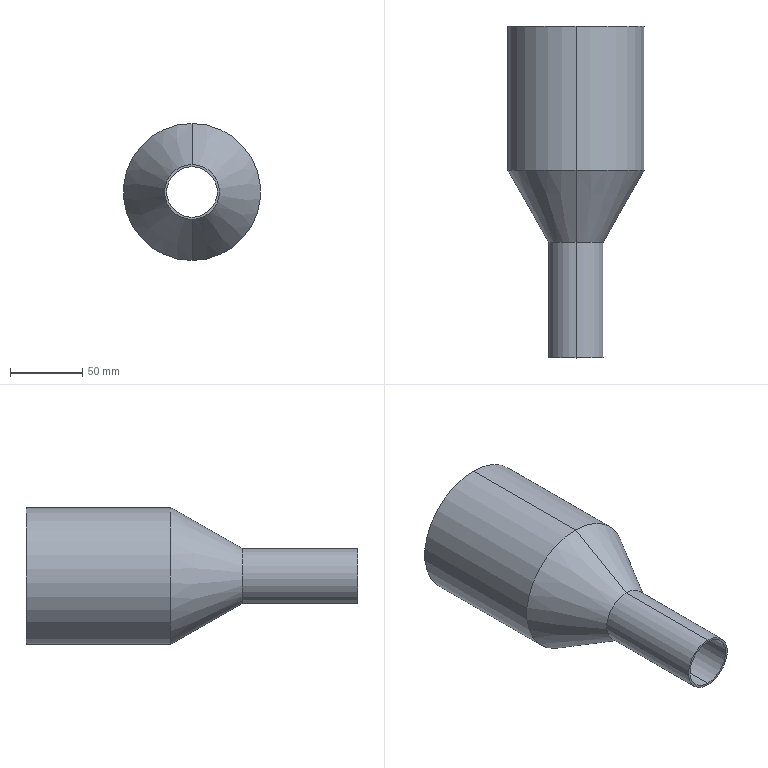Part | SolidWorks | features BaseBody 1 | 1 solid | 14 faces | box 95 x 230 x 95 mm | volume 75396 mm3 | cylinder 8 | cone 4 | plane 2 | commonest cylinder face diameters 35 x2 38 x2 92 x2 95 x2
STEP:
#1=CARTESIAN_POINT('',(0.,130.,47.5));
#2=VERTEX_POINT('',#1);
#3=CARTESIAN_POINT('',(0.,130.,-47.5));
#4=VERTEX_POINT('',#3);
#5=CARTESIAN_POINT('',(0.,130.,0.));
#6=DIRECTION('',(0.,1.,0.));
#7=DIRECTION('',(0.,0.,1.));
#8=AXIS2_PLACEMENT_3D('',#5,#6,#7);
#9=CIRCLE('',#8,47.5);
#10=EDGE_CURVE('',#2,#4,#9,.T.);
#11=ORIENTED_EDGE('',*,*,#10,.T.);
#12=CARTESIAN_POINT('',(0.,230.,-47.5));
#13=VERTEX_POINT('',#12);
#14=CARTESIAN_POINT('',(0.,119.95,-47.5));
#15=DIRECTION('',(0.,1.,0.));
#16=VECTOR('',#15,1000.);
#17=LINE('',#14,#16);
#18=EDGE_CURVE('',#4,#13,#17,.T.);
#19=ORIENTED_EDGE('',*,*,#18,.T.);
#20=CARTESIAN_POINT('',(0.,230.,47.5));
#21=VERTEX_POINT('',#20);
#22=CARTESIAN_POINT('',(0.,230.,0.));
#23=DIRECTION('',(0.,1.,0.));
#24=DIRECTION('',(0.,0.,1.));
#25=AXIS2_PLACEMENT_3D('',#22,#23,#24);
#26=CIRCLE('',#25,47.5);
#27=EDGE_CURVE('',#21,#13,#26,.T.);
#28=ORIENTED_EDGE('',*,*,#27,.F.);
#29=CARTESIAN_POINT('',(0.,119.95,47.5));
#30=DIRECTION('',(0.,1.,0.));
#31=VECTOR('',#30,1000.);
#32=LINE('',#29,#31);
#33=EDGE_CURVE('',#2,#21,#32,.T.);
#34=ORIENTED_EDGE('',*,*,#33,.F.);
#35=EDGE_LOOP('',(#11,#19,#28,#34));
#36=FACE_OUTER_BOUND('',#35,.T.);
#37=CARTESIAN_POINT('',(0.,119.95,0.));
#38=DIRECTION('',(0.,1.,0.));
#39=DIRECTION('',(0.,0.,1.));
#40=AXIS2_PLACEMENT_3D('',#37,#38,#39);
#41=CYLINDRICAL_SURFACE('',#40,47.5);
#42=ADVANCED_FACE('',(#36),#41,.T.);
#43=CARTESIAN_POINT('',(0.,80.,19.));
#44=VERTEX_POINT('',#43);
#45=CARTESIAN_POINT('',(0.,80.,-19.));
#46=VERTEX_POINT('',#45);
#47=CARTESIAN_POINT('',(0.,80.,0.));
#48=DIRECTION('',(0.,1.,0.));
#49=DIRECTION('',(0.,0.,1.));
#50=AXIS2_PLACEMENT_3D('',#47,#48,#49);
#51=CIRCLE('',#50,19.);
#52=EDGE_CURVE('',#44,#46,#51,.T.);
#53=ORIENTED_EDGE('',*,*,#52,.T.);
#54=CARTESIAN_POINT('',(0.,80.,-19.));
#55=DIRECTION('',(0.,0.8688,-0.4952));
#56=VECTOR('',#55,1000.);
#57=LINE('',#54,#56);
#58=EDGE_CURVE('',#46,#4,#57,.T.);
#59=ORIENTED_EDGE('',*,*,#58,.T.);
#60=ORIENTED_EDGE('',*,*,#10,.F.);
#61=CARTESIAN_POINT('',(0.,80.,19.));
#62=DIRECTION('',(0.,0.8688,0.4952));
#63=VECTOR('',#62,1000.);
#64=LINE('',#61,#63);
#65=EDGE_CURVE('',#44,#2,#64,.T.);
#66=ORIENTED_EDGE('',*,*,#65,.F.);
#67=EDGE_LOOP('',(#53,#59,#60,#66));
#68=FACE_OUTER_BOUND('',#67,.T.);
#69=CARTESIAN_POINT('',(0.,80.,0.));
#70=DIRECTION('',(0.,1.,0.));
#71=DIRECTION('',(0.,0.,1.));
#72=AXIS2_PLACEMENT_3D('',#69,#70,#71);
#73=CONICAL_SURFACE('',#72,19.,0.5181);
#74=ADVANCED_FACE('',(#68),#73,.T.);
#75=CARTESIAN_POINT('',(0.,0.,19.));
#76=VERTEX_POINT('',#75);
#77=CARTESIAN_POINT('',(0.,0.,-19.));
#78=VERTEX_POINT('',#77);
#79=CARTESIAN_POINT('',(0.,0.,0.));
#80=DIRECTION('',(0.,1.,0.));
#81=DIRECTION('',(0.,0.,1.));
#82=AXIS2_PLACEMENT_3D('',#79,#80,#81);
#83=CIRCLE('',#82,19.);
#84=EDGE_CURVE('',#76,#78,#83,.T.);
#85=ORIENTED_EDGE('',*,*,#84,.T.);
#86=CARTESIAN_POINT('',(0.,119.95,-19.));
#87=DIRECTION('',(0.,1.,0.));
#88=VECTOR('',#87,1000.);
#89=LINE('',#86,#88);
#90=EDGE_CURVE('',#78,#46,#89,.T.);
#91=ORIENTED_EDGE('',*,*,#90,.T.);
#92=ORIENTED_EDGE('',*,*,#52,.F.);
#93=CARTESIAN_POINT('',(0.,119.95,19.));
#94=DIRECTION('',(0.,1.,0.));
#95=VECTOR('',#94,1000.);
#96=LINE('',#93,#95);
#97=EDGE_CURVE('',#76,#44,#96,.T.);
#98=ORIENTED_EDGE('',*,*,#97,.F.);
#99=EDGE_LOOP('',(#85,#91,#92,#98));
#100=FACE_OUTER_BOUND('',#99,.T.);
#101=CARTESIAN_POINT('',(0.,119.95,0.));
#102=DIRECTION('',(0.,1.,0.));
#103=DIRECTION('',(0.,0.,1.));
#104=AXIS2_PLACEMENT_3D('',#101,#102,#103);
#105=CYLINDRICAL_SURFACE('',#104,19.);
#106=ADVANCED_FACE('',(#100),#105,.T.);
#107=CARTESIAN_POINT('',(0.,0.,-17.5));
#108=VERTEX_POINT('',#107);
#109=CARTESIAN_POINT('',(0.,0.,17.5));
#110=VERTEX_POINT('',#109);
#111=CARTESIAN_POINT('',(0.,0.,0.));
#112=DIRECTION('',(0.,1.,0.));
#113=DIRECTION('',(0.,0.,1.));
#114=AXIS2_PLACEMENT_3D('',#111,#112,#113);
#115=CIRCLE('',#114,17.5);
#116=EDGE_CURVE('',#108,#110,#115,.T.);
#117=ORIENTED_EDGE('',*,*,#116,.F.);
#118=CARTESIAN_POINT('',(0.,80.397,-17.5));
#119=VERTEX_POINT('',#118);
#120=CARTESIAN_POINT('',(0.,119.95,-17.5));
#121=DIRECTION('',(0.,1.,0.));
#122=VECTOR('',#121,1000.);
#123=LINE('',#120,#122);
#124=EDGE_CURVE('',#108,#119,#123,.T.);
#125=ORIENTED_EDGE('',*,*,#124,.T.);
#126=CARTESIAN_POINT('',(0.,80.397,17.5));
#127=VERTEX_POINT('',#126);
#128=CARTESIAN_POINT('',(0.,80.397,0.));
#129=DIRECTION('',(0.,1.,0.));
#130=DIRECTION('',(0.,0.,1.));
#131=AXIS2_PLACEMENT_3D('',#128,#129,#130);
#132=CIRCLE('',#131,17.5);
#133=EDGE_CURVE('',#119,#127,#132,.T.);
#134=ORIENTED_EDGE('',*,*,#133,.T.);
#135=CARTESIAN_POINT('',(0.,119.95,17.5));
#136=DIRECTION('',(0.,1.,0.));
#137=VECTOR('',#136,1000.);
#138=LINE('',#135,#137);
#139=EDGE_CURVE('',#110,#127,#138,.T.);
#140=ORIENTED_EDGE('',*,*,#139,.F.);
#141=EDGE_LOOP('',(#117,#125,#134,#140));
#142=FACE_OUTER_BOUND('',#141,.T.);
#143=CARTESIAN_POINT('',(0.,119.95,0.));
#144=DIRECTION('',(0.,1.,0.));
#145=DIRECTION('',(0.,0.,1.));
#146=AXIS2_PLACEMENT_3D('',#143,#144,#145);
#147=CYLINDRICAL_SURFACE('',#146,17.5);
#148=ADVANCED_FACE('',(#142),#147,.F.);
#149=ORIENTED_EDGE('',*,*,#133,.F.);
#150=CARTESIAN_POINT('',(0.,130.397,-46.));
#151=VERTEX_POINT('',#150);
#152=CARTESIAN_POINT('',(0.,80.397,-17.5));
#153=DIRECTION('',(0.,0.8688,-0.4952));
#154=VECTOR('',#153,1000.);
#155=LINE('',#152,#154);
#156=EDGE_CURVE('',#119,#151,#155,.T.);
#157=ORIENTED_EDGE('',*,*,#156,.T.);
#158=CARTESIAN_POINT('',(0.,130.397,46.));
#159=VERTEX_POINT('',#158);
#160=CARTESIAN_POINT('',(0.,130.397,0.));
#161=DIRECTION('',(0.,1.,0.));
#162=DIRECTION('',(0.,0.,1.));
#163=AXIS2_PLACEMENT_3D('',#160,#161,#162);
#164=CIRCLE('',#163,46.);
#165=EDGE_CURVE('',#151,#159,#164,.T.);
#166=ORIENTED_EDGE('',*,*,#165,.T.);
#167=CARTESIAN_POINT('',(0.,80.397,17.5));
#168=DIRECTION('',(0.,0.8688,0.4952));
#169=VECTOR('',#168,1000.);
#170=LINE('',#167,#169);
#171=EDGE_CURVE('',#127,#159,#170,.T.);
#172=ORIENTED_EDGE('',*,*,#171,.F.);
#173=EDGE_LOOP('',(#149,#157,#166,#172));
#174=FACE_OUTER_BOUND('',#173,.T.);
#175=CARTESIAN_POINT('',(0.,80.397,0.));
#176=DIRECTION('',(0.,1.,0.));
#177=DIRECTION('',(0.,0.,1.));
#178=AXIS2_PLACEMENT_3D('',#175,#176,#177);
#179=CONICAL_SURFACE('',#178,17.5,0.5181);
#180=ADVANCED_FACE('',(#174),#179,.F.);
#181=ORIENTED_EDGE('',*,*,#165,.F.);
#182=CARTESIAN_POINT('',(0.,230.,-46.));
#183=VERTEX_POINT('',#182);
#184=CARTESIAN_POINT('',(0.,119.95,-46.));
#185=DIRECTION('',(0.,1.,0.));
#186=VECTOR('',#185,1000.);
#187=LINE('',#184,#186);
#188=EDGE_CURVE('',#151,#183,#187,.T.);
#189=ORIENTED_EDGE('',*,*,#188,.T.);
#190=CARTESIAN_POINT('',(0.,230.,46.));
#191=VERTEX_POINT('',#190);
#192=CARTESIAN_POINT('',(0.,230.,0.));
#193=DIRECTION('',(0.,1.,0.));
#194=DIRECTION('',(0.,0.,1.));
#195=AXIS2_PLACEMENT_3D('',#192,#193,#194);
#196=CIRCLE('',#195,46.);
#197=EDGE_CURVE('',#183,#191,#196,.T.);
#198=ORIENTED_EDGE('',*,*,#197,.T.);
#199=CARTESIAN_POINT('',(0.,119.95,46.));
#200=DIRECTION('',(0.,1.,0.));
#201=VECTOR('',#200,1000.);
#202=LINE('',#199,#201);
#203=EDGE_CURVE('',#159,#191,#202,.T.);
#204=ORIENTED_EDGE('',*,*,#203,.F.);
#205=EDGE_LOOP('',(#181,#189,#198,#204));
#206=FACE_OUTER_BOUND('',#205,.T.);
#207=CARTESIAN_POINT('',(0.,119.95,0.));
#208=DIRECTION('',(0.,1.,0.));
#209=DIRECTION('',(0.,0.,1.));
#210=AXIS2_PLACEMENT_3D('',#207,#208,#209);
#211=CYLINDRICAL_SURFACE('',#210,46.);
#212=ADVANCED_FACE('',(#206),#211,.F.);
#213=CARTESIAN_POINT('',(0.,230.,0.));
#214=DIRECTION('',(0.,1.,0.));
#215=DIRECTION('',(0.,0.,1.));
#216=AXIS2_PLACEMENT_3D('',#213,#214,#215);
#217=CIRCLE('',#216,46.);
#218=EDGE_CURVE('',#191,#183,#217,.T.);
#219=ORIENTED_EDGE('',*,*,#218,.F.);
#220=ORIENTED_EDGE('',*,*,#197,.F.);
#221=EDGE_LOOP('',(#219,#220));
#222=FACE_BOUND('',#221,.T.);
#223=ORIENTED_EDGE('',*,*,#27,.T.);
#224=CARTESIAN_POINT('',(0.,230.,0.));
#225=DIRECTION('',(0.,1.,0.));
#226=DIRECTION('',(0.,0.,1.));
#227=AXIS2_PLACEMENT_3D('',#224,#225,#226);
#228=CIRCLE('',#227,47.5);
#229=EDGE_CURVE('',#13,#21,#228,.T.);
#230=ORIENTED_EDGE('',*,*,#229,.T.);
#231=EDGE_LOOP('',(#223,#230));
#232=FACE_OUTER_BOUND('',#231,.T.);
#233=CARTESIAN_POINT('',(0.,230.,47.5));
#234=DIRECTION('',(0.,-1.,0.));
#235=DIRECTION('',(0.,0.,-1.));
#236=AXIS2_PLACEMENT_3D('',#233,#234,#235);
#237=PLANE('',#236);
#238=ADVANCED_FACE('',(#222,#232),#237,.F.);
#239=CARTESIAN_POINT('',(0.,0.,0.));
#240=DIRECTION('',(0.,1.,0.));
#241=DIRECTION('',(0.,0.,1.));
#242=AXIS2_PLACEMENT_3D('',#239,#240,#241);
#243=CIRCLE('',#242,17.5);
#244=EDGE_CURVE('',#110,#108,#243,.T.);
#245=ORIENTED_EDGE('',*,*,#244,.T.);
#246=ORIENTED_EDGE('',*,*,#116,.T.);
#247=EDGE_LOOP('',(#245,#246));
#248=FACE_BOUND('',#247,.T.);
#249=ORIENTED_EDGE('',*,*,#84,.F.);
#250=CARTESIAN_POINT('',(0.,0.,0.));
#251=DIRECTION('',(0.,1.,0.));
#252=DIRECTION('',(0.,0.,1.));
#253=AXIS2_PLACEMENT_3D('',#250,#251,#252);
#254=CIRCLE('',#253,19.);
#255=EDGE_CURVE('',#78,#76,#254,.T.);
#256=ORIENTED_EDGE('',*,*,#255,.F.);
#257=EDGE_LOOP('',(#249,#256));
#258=FACE_OUTER_BOUND('',#257,.T.);
#259=CARTESIAN_POINT('',(0.,0.,17.5));
#260=DIRECTION('',(0.,1.,0.));
#261=DIRECTION('',(1.,0.,0.));
#262=AXIS2_PLACEMENT_3D('',#259,#260,#261);
#263=PLANE('',#262);
#264=ADVANCED_FACE('',(#248,#258),#263,.F.);
#265=ORIENTED_EDGE('',*,*,#188,.F.);
#266=CARTESIAN_POINT('',(0.,130.397,0.));
#267=DIRECTION('',(0.,1.,0.));
#268=DIRECTION('',(0.,0.,1.));
#269=AXIS2_PLACEMENT_3D('',#266,#267,#268);
#270=CIRCLE('',#269,46.);
#271=EDGE_CURVE('',#159,#151,#270,.T.);
#272=ORIENTED_EDGE('',*,*,#271,.F.);
#273=ORIENTED_EDGE('',*,*,#203,.T.);
#274=ORIENTED_EDGE('',*,*,#218,.T.);
#275=EDGE_LOOP('',(#265,#272,#273,#274));
#276=FACE_OUTER_BOUND('',#275,.T.);
#277=CARTESIAN_POINT('',(0.,119.95,0.));
#278=DIRECTION('',(0.,1.,0.));
#279=DIRECTION('',(0.,0.,1.));
#280=AXIS2_PLACEMENT_3D('',#277,#278,#279);
#281=CYLINDRICAL_SURFACE('',#280,46.);
#282=ADVANCED_FACE('',(#276),#281,.F.);
#283=ORIENTED_EDGE('',*,*,#156,.F.);
#284=CARTESIAN_POINT('',(0.,80.397,0.));
#285=DIRECTION('',(0.,1.,0.));
#286=DIRECTION('',(0.,0.,1.));
#287=AXIS2_PLACEMENT_3D('',#284,#285,#286);
#288=CIRCLE('',#287,17.5);
#289=EDGE_CURVE('',#127,#119,#288,.T.);
#290=ORIENTED_EDGE('',*,*,#289,.F.);
#291=ORIENTED_EDGE('',*,*,#171,.T.);
#292=ORIENTED_EDGE('',*,*,#271,.T.);
#293=EDGE_LOOP('',(#283,#290,#291,#292));
#294=FACE_OUTER_BOUND('',#293,.T.);
#295=CARTESIAN_POINT('',(0.,80.397,0.));
#296=DIRECTION('',(0.,1.,0.));
#297=DIRECTION('',(0.,0.,1.));
#298=AXIS2_PLACEMENT_3D('',#295,#296,#297);
#299=CONICAL_SURFACE('',#298,17.5,0.5181);
#300=ADVANCED_FACE('',(#294),#299,.F.);
#301=ORIENTED_EDGE('',*,*,#124,.F.);
#302=ORIENTED_EDGE('',*,*,#244,.F.);
#303=ORIENTED_EDGE('',*,*,#139,.T.);
#304=ORIENTED_EDGE('',*,*,#289,.T.);
#305=EDGE_LOOP('',(#301,#302,#303,#304));
#306=FACE_OUTER_BOUND('',#305,.T.);
#307=CARTESIAN_POINT('',(0.,119.95,0.));
#308=DIRECTION('',(0.,1.,0.));
#309=DIRECTION('',(0.,0.,1.));
#310=AXIS2_PLACEMENT_3D('',#307,#308,#309);
#311=CYLINDRICAL_SURFACE('',#310,17.5);
#312=ADVANCED_FACE('',(#306),#311,.F.);
#313=ORIENTED_EDGE('',*,*,#90,.F.);
#314=ORIENTED_EDGE('',*,*,#255,.T.);
#315=ORIENTED_EDGE('',*,*,#97,.T.);
#316=CARTESIAN_POINT('',(0.,80.,0.));
#317=DIRECTION('',(0.,1.,0.));
#318=DIRECTION('',(0.,0.,1.));
#319=AXIS2_PLACEMENT_3D('',#316,#317,#318);
#320=CIRCLE('',#319,19.);
#321=EDGE_CURVE('',#46,#44,#320,.T.);
#322=ORIENTED_EDGE('',*,*,#321,.F.);
#323=EDGE_LOOP('',(#313,#314,#315,#322));
#324=FACE_OUTER_BOUND('',#323,.T.);
#325=CARTESIAN_POINT('',(0.,119.95,0.));
#326=DIRECTION('',(0.,1.,0.));
#327=DIRECTION('',(0.,0.,1.));
#328=AXIS2_PLACEMENT_3D('',#325,#326,#327);
#329=CYLINDRICAL_SURFACE('',#328,19.);
#330=ADVANCED_FACE('',(#324),#329,.T.);
#331=ORIENTED_EDGE('',*,*,#58,.F.);
#332=ORIENTED_EDGE('',*,*,#321,.T.);
#333=ORIENTED_EDGE('',*,*,#65,.T.);
#334=CARTESIAN_POINT('',(0.,130.,0.));
#335=DIRECTION('',(0.,1.,0.));
#336=DIRECTION('',(0.,0.,1.));
#337=AXIS2_PLACEMENT_3D('',#334,#335,#336);
#338=CIRCLE('',#337,47.5);
#339=EDGE_CURVE('',#4,#2,#338,.T.);
#340=ORIENTED_EDGE('',*,*,#339,.F.);
#341=EDGE_LOOP('',(#331,#332,#333,#340));
#342=FACE_OUTER_BOUND('',#341,.T.);
#343=CARTESIAN_POINT('',(0.,80.,0.));
#344=DIRECTION('',(0.,1.,0.));
#345=DIRECTION('',(0.,0.,1.));
#346=AXIS2_PLACEMENT_3D('',#343,#344,#345);
#347=CONICAL_SURFACE('',#346,19.,0.5181);
#348=ADVANCED_FACE('',(#342),#347,.T.);
#349=ORIENTED_EDGE('',*,*,#18,.F.);
#350=ORIENTED_EDGE('',*,*,#339,.T.);
#351=ORIENTED_EDGE('',*,*,#33,.T.);
#352=ORIENTED_EDGE('',*,*,#229,.F.);
#353=EDGE_LOOP('',(#349,#350,#351,#352));
#354=FACE_OUTER_BOUND('',#353,.T.);
#355=CARTESIAN_POINT('',(0.,119.95,0.));
#356=DIRECTION('',(0.,1.,0.));
#357=DIRECTION('',(0.,0.,1.));
#358=AXIS2_PLACEMENT_3D('',#355,#356,#357);
#359=CYLINDRICAL_SURFACE('',#358,47.5);
#360=ADVANCED_FACE('',(#354),#359,.T.);
#361=CLOSED_SHELL('',(#42,#74,#106,#148,#180,#212,#238,#264,#282,#300,#312,#330,#348,#360));
#362=MANIFOLD_SOLID_BREP('',#361);
#363=CARTESIAN_POINT('',(0.,0.,0.));
#364=DIRECTION('',(0.,0.,1.));
#365=DIRECTION('',(1.,0.,0.));
#366=AXIS2_PLACEMENT_3D('',#363,#364,#365);
#367=(LENGTH_UNIT()NAMED_UNIT(*)SI_UNIT(.MILLI.,.METRE.));
#368=UNCERTAINTY_MEASURE_WITH_UNIT(LENGTH_MEASURE(0.00001),#367,'','');
#369=(NAMED_UNIT(*)PLANE_ANGLE_UNIT()SI_UNIT($,.RADIAN.));
#370=(NAMED_UNIT(*)SI_UNIT($,.STERADIAN.)SOLID_ANGLE_UNIT());
#371=(GEOMETRIC_REPRESENTATION_CONTEXT(3)GLOBAL_UNCERTAINTY_ASSIGNED_CONTEXT((#368))GLOBAL_UNIT_ASSIGNED_CONTEXT((#367,#369,#370))REPRESENTATION_CONTEXT('',''));
#372=ADVANCED_BREP_SHAPE_REPRESENTATION('',(#362,#366),#371);